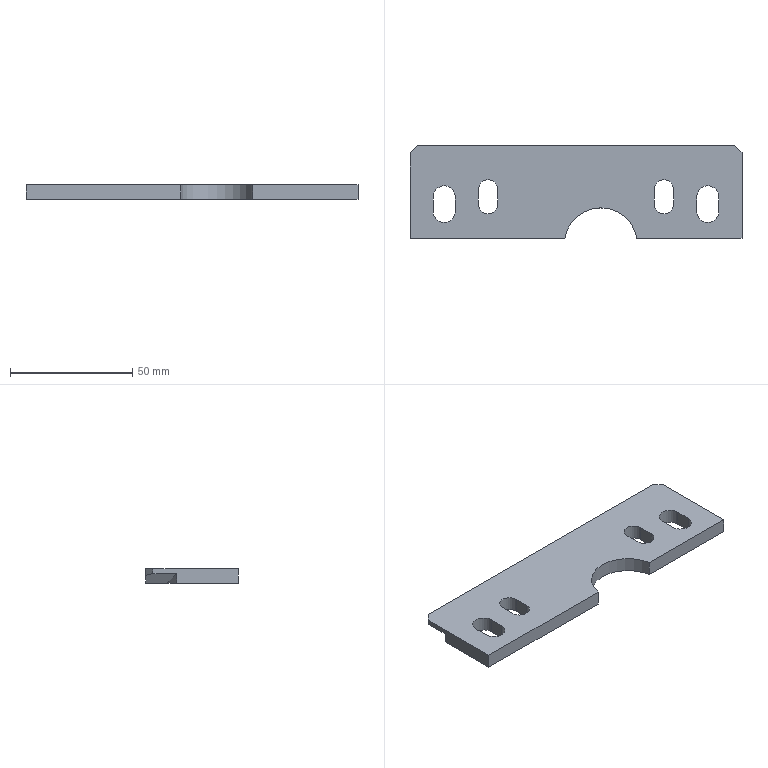Part | STEP file | gslz 2016.10.28-13_id710_x_t | 1 solid | 31 faces | box 136 x 38 x 6 mm | volume 26219 mm3 | plane 22 | cylinder 9 | commonest cylinder face diameters 8 x4 9 x4 30 x1